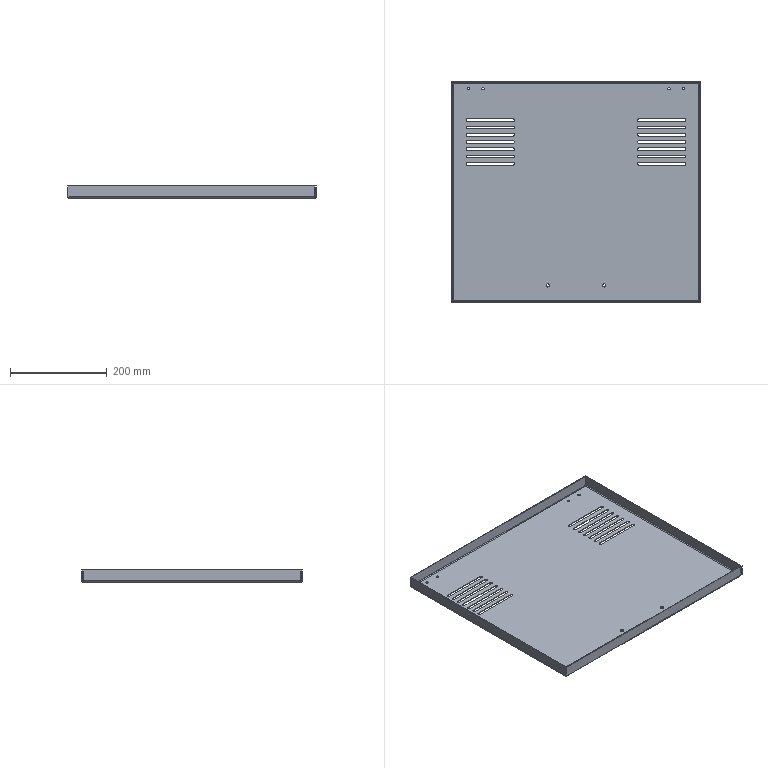Part | STEP file | SynoNew-0304-053 | 1 solid | 104 faces | box 515 x 457 x 25 mm | volume 405617 mm3 | plane 62 | cylinder 42 | commonest cylinder face diameters 6 x32 3 x4 4.917 x4 6.647 x2